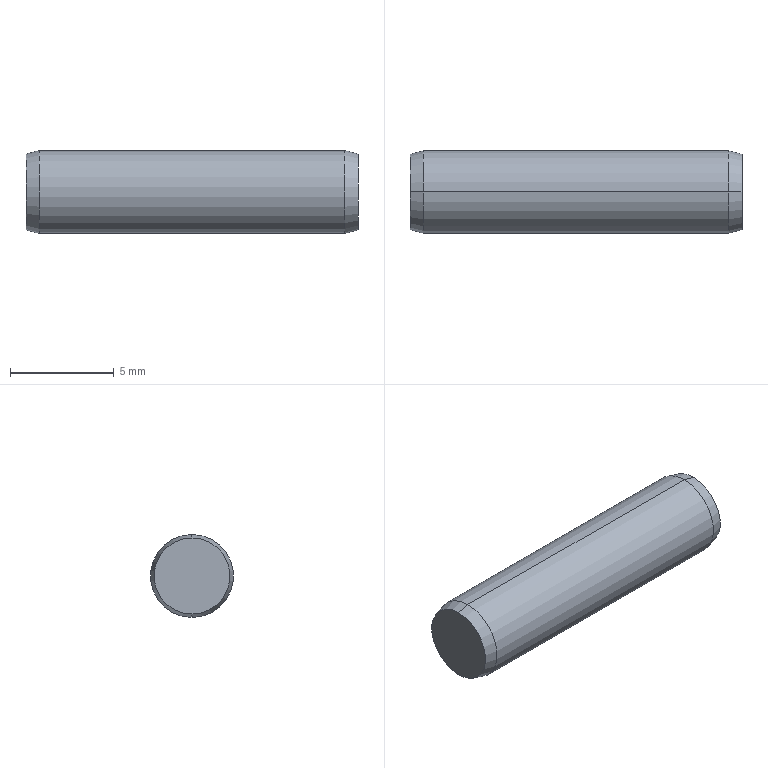Part | SolidWorks | features Revolution 1 | 1 solid | 8 faces | box 16 x 4 x 4 mm | volume 199.763 mm3 | cone 4 | cylinder 2 | plane 2 | commonest cylinder face diameters 4 x2
STEP:
#1=CARTESIAN_POINT('',(13.74,0.,2.));
#2=VERTEX_POINT('',#1);
#3=CARTESIAN_POINT('',(13.74,0.,-2.));
#4=VERTEX_POINT('',#3);
#5=CARTESIAN_POINT('',(13.74,0.,0.));
#6=DIRECTION('',(-1.,0.,0.));
#7=DIRECTION('',(0.,0.,1.));
#8=AXIS2_PLACEMENT_3D('',#5,#6,#7);
#9=CIRCLE('',#8,2.);
#10=EDGE_CURVE('',#2,#4,#9,.T.);
#11=ORIENTED_EDGE('',*,*,#10,.T.);
#12=CARTESIAN_POINT('',(-1.,0.,-2.));
#13=VERTEX_POINT('',#12);
#14=CARTESIAN_POINT('',(0.,0.,-2.));
#15=DIRECTION('',(-1.,0.,0.));
#16=VECTOR('',#15,1000.);
#17=LINE('',#14,#16);
#18=EDGE_CURVE('',#4,#13,#17,.T.);
#19=ORIENTED_EDGE('',*,*,#18,.T.);
#20=CARTESIAN_POINT('',(-1.,0.,2.));
#21=VERTEX_POINT('',#20);
#22=CARTESIAN_POINT('',(-1.,0.,0.));
#23=DIRECTION('',(-1.,0.,0.));
#24=DIRECTION('',(0.,0.,1.));
#25=AXIS2_PLACEMENT_3D('',#22,#23,#24);
#26=CIRCLE('',#25,2.);
#27=EDGE_CURVE('',#21,#13,#26,.T.);
#28=ORIENTED_EDGE('',*,*,#27,.F.);
#29=CARTESIAN_POINT('',(0.,0.,2.));
#30=DIRECTION('',(-1.,0.,0.));
#31=VECTOR('',#30,1000.);
#32=LINE('',#29,#31);
#33=EDGE_CURVE('',#2,#21,#32,.T.);
#34=ORIENTED_EDGE('',*,*,#33,.F.);
#35=EDGE_LOOP('',(#11,#19,#28,#34));
#36=FACE_OUTER_BOUND('',#35,.T.);
#37=CARTESIAN_POINT('',(0.,0.,0.));
#38=DIRECTION('',(-1.,0.,0.));
#39=DIRECTION('',(0.,0.,1.));
#40=AXIS2_PLACEMENT_3D('',#37,#38,#39);
#41=CYLINDRICAL_SURFACE('',#40,2.);
#42=ADVANCED_FACE('',(#36),#41,.T.);
#43=CARTESIAN_POINT('',(-1.63,0.,1.831));
#44=VERTEX_POINT('',#43);
#45=CARTESIAN_POINT('',(-1.63,0.,-1.831));
#46=VERTEX_POINT('',#45);
#47=CARTESIAN_POINT('',(-1.63,0.,0.));
#48=DIRECTION('',(-1.,0.,0.));
#49=DIRECTION('',(0.,0.,1.));
#50=AXIS2_PLACEMENT_3D('',#47,#48,#49);
#51=CIRCLE('',#50,1.831);
#52=EDGE_CURVE('',#44,#46,#51,.T.);
#53=ORIENTED_EDGE('',*,*,#52,.F.);
#54=CARTESIAN_POINT('',(-1.,0.,2.));
#55=DIRECTION('',(0.9659,0.,0.2588));
#56=VECTOR('',#55,1000.);
#57=LINE('',#54,#56);
#58=EDGE_CURVE('',#44,#21,#57,.T.);
#59=ORIENTED_EDGE('',*,*,#58,.T.);
#60=ORIENTED_EDGE('',*,*,#27,.T.);
#61=CARTESIAN_POINT('',(-1.,0.,-2.));
#62=DIRECTION('',(0.9659,0.,-0.2588));
#63=VECTOR('',#62,1000.);
#64=LINE('',#61,#63);
#65=EDGE_CURVE('',#46,#13,#64,.T.);
#66=ORIENTED_EDGE('',*,*,#65,.F.);
#67=EDGE_LOOP('',(#53,#59,#60,#66));
#68=FACE_OUTER_BOUND('',#67,.T.);
#69=CARTESIAN_POINT('',(-1.,0.,0.));
#70=DIRECTION('',(1.,0.,0.));
#71=DIRECTION('',(0.,0.,-1.));
#72=AXIS2_PLACEMENT_3D('',#69,#70,#71);
#73=CONICAL_SURFACE('',#72,2.,0.2618);
#74=ADVANCED_FACE('',(#68),#73,.T.);
#75=CARTESIAN_POINT('',(14.37,0.,1.831));
#76=VERTEX_POINT('',#75);
#77=CARTESIAN_POINT('',(14.37,0.,-1.831));
#78=VERTEX_POINT('',#77);
#79=CARTESIAN_POINT('',(14.37,0.,0.));
#80=DIRECTION('',(-1.,0.,0.));
#81=DIRECTION('',(0.,0.,1.));
#82=AXIS2_PLACEMENT_3D('',#79,#80,#81);
#83=CIRCLE('',#82,1.831);
#84=EDGE_CURVE('',#76,#78,#83,.T.);
#85=ORIENTED_EDGE('',*,*,#84,.T.);
#86=CARTESIAN_POINT('',(14.37,0.,-1.831));
#87=DIRECTION('',(-0.9659,0.,-0.2588));
#88=VECTOR('',#87,1000.);
#89=LINE('',#86,#88);
#90=EDGE_CURVE('',#78,#4,#89,.T.);
#91=ORIENTED_EDGE('',*,*,#90,.T.);
#92=ORIENTED_EDGE('',*,*,#10,.F.);
#93=CARTESIAN_POINT('',(14.37,0.,1.831));
#94=DIRECTION('',(-0.9659,0.,0.2588));
#95=VECTOR('',#94,1000.);
#96=LINE('',#93,#95);
#97=EDGE_CURVE('',#76,#2,#96,.T.);
#98=ORIENTED_EDGE('',*,*,#97,.F.);
#99=EDGE_LOOP('',(#85,#91,#92,#98));
#100=FACE_OUTER_BOUND('',#99,.T.);
#101=CARTESIAN_POINT('',(14.37,0.,0.));
#102=DIRECTION('',(-1.,0.,0.));
#103=DIRECTION('',(0.,0.,1.));
#104=AXIS2_PLACEMENT_3D('',#101,#102,#103);
#105=CONICAL_SURFACE('',#104,1.831,0.2618);
#106=ADVANCED_FACE('',(#100),#105,.T.);
#107=ORIENTED_EDGE('',*,*,#90,.F.);
#108=CARTESIAN_POINT('',(14.37,0.,0.));
#109=DIRECTION('',(-1.,0.,0.));
#110=DIRECTION('',(0.,0.,1.));
#111=AXIS2_PLACEMENT_3D('',#108,#109,#110);
#112=CIRCLE('',#111,1.831);
#113=EDGE_CURVE('',#78,#76,#112,.T.);
#114=ORIENTED_EDGE('',*,*,#113,.T.);
#115=ORIENTED_EDGE('',*,*,#97,.T.);
#116=CARTESIAN_POINT('',(13.74,0.,0.));
#117=DIRECTION('',(-1.,0.,0.));
#118=DIRECTION('',(0.,0.,1.));
#119=AXIS2_PLACEMENT_3D('',#116,#117,#118);
#120=CIRCLE('',#119,2.);
#121=EDGE_CURVE('',#4,#2,#120,.T.);
#122=ORIENTED_EDGE('',*,*,#121,.F.);
#123=EDGE_LOOP('',(#107,#114,#115,#122));
#124=FACE_OUTER_BOUND('',#123,.T.);
#125=CARTESIAN_POINT('',(14.37,0.,0.));
#126=DIRECTION('',(-1.,0.,0.));
#127=DIRECTION('',(0.,0.,1.));
#128=AXIS2_PLACEMENT_3D('',#125,#126,#127);
#129=CONICAL_SURFACE('',#128,1.831,0.2618);
#130=ADVANCED_FACE('',(#124),#129,.T.);
#131=ORIENTED_EDGE('',*,*,#84,.F.);
#132=ORIENTED_EDGE('',*,*,#113,.F.);
#133=EDGE_LOOP('',(#131,#132));
#134=FACE_OUTER_BOUND('',#133,.T.);
#135=CARTESIAN_POINT('',(14.37,1.831,0.));
#136=DIRECTION('',(-1.,0.,0.));
#137=DIRECTION('',(0.,0.,1.));
#138=AXIS2_PLACEMENT_3D('',#135,#136,#137);
#139=PLANE('',#138);
#140=ADVANCED_FACE('',(#134),#139,.F.);
#141=CARTESIAN_POINT('',(-1.63,0.,0.));
#142=DIRECTION('',(-1.,0.,0.));
#143=DIRECTION('',(0.,0.,1.));
#144=AXIS2_PLACEMENT_3D('',#141,#142,#143);
#145=CIRCLE('',#144,1.831);
#146=EDGE_CURVE('',#46,#44,#145,.T.);
#147=ORIENTED_EDGE('',*,*,#146,.T.);
#148=ORIENTED_EDGE('',*,*,#52,.T.);
#149=EDGE_LOOP('',(#147,#148));
#150=FACE_OUTER_BOUND('',#149,.T.);
#151=CARTESIAN_POINT('',(-1.63,1.831,0.));
#152=DIRECTION('',(1.,0.,0.));
#153=DIRECTION('',(0.,0.,-1.));
#154=AXIS2_PLACEMENT_3D('',#151,#152,#153);
#155=PLANE('',#154);
#156=ADVANCED_FACE('',(#150),#155,.F.);
#157=ORIENTED_EDGE('',*,*,#58,.F.);
#158=ORIENTED_EDGE('',*,*,#146,.F.);
#159=ORIENTED_EDGE('',*,*,#65,.T.);
#160=CARTESIAN_POINT('',(-1.,0.,0.));
#161=DIRECTION('',(-1.,0.,0.));
#162=DIRECTION('',(0.,0.,1.));
#163=AXIS2_PLACEMENT_3D('',#160,#161,#162);
#164=CIRCLE('',#163,2.);
#165=EDGE_CURVE('',#13,#21,#164,.T.);
#166=ORIENTED_EDGE('',*,*,#165,.T.);
#167=EDGE_LOOP('',(#157,#158,#159,#166));
#168=FACE_OUTER_BOUND('',#167,.T.);
#169=CARTESIAN_POINT('',(-1.,0.,0.));
#170=DIRECTION('',(1.,0.,0.));
#171=DIRECTION('',(0.,0.,-1.));
#172=AXIS2_PLACEMENT_3D('',#169,#170,#171);
#173=CONICAL_SURFACE('',#172,2.,0.2618);
#174=ADVANCED_FACE('',(#168),#173,.T.);
#175=ORIENTED_EDGE('',*,*,#18,.F.);
#176=ORIENTED_EDGE('',*,*,#121,.T.);
#177=ORIENTED_EDGE('',*,*,#33,.T.);
#178=ORIENTED_EDGE('',*,*,#165,.F.);
#179=EDGE_LOOP('',(#175,#176,#177,#178));
#180=FACE_OUTER_BOUND('',#179,.T.);
#181=CARTESIAN_POINT('',(0.,0.,0.));
#182=DIRECTION('',(-1.,0.,0.));
#183=DIRECTION('',(0.,0.,1.));
#184=AXIS2_PLACEMENT_3D('',#181,#182,#183);
#185=CYLINDRICAL_SURFACE('',#184,2.);
#186=ADVANCED_FACE('',(#180),#185,.T.);
#187=CLOSED_SHELL('',(#42,#74,#106,#130,#140,#156,#174,#186));
#188=MANIFOLD_SOLID_BREP('',#187);
#189=CARTESIAN_POINT('',(0.,0.,0.));
#190=DIRECTION('',(0.,0.,1.));
#191=DIRECTION('',(1.,0.,0.));
#192=AXIS2_PLACEMENT_3D('',#189,#190,#191);
#193=(LENGTH_UNIT()NAMED_UNIT(*)SI_UNIT(.MILLI.,.METRE.));
#194=UNCERTAINTY_MEASURE_WITH_UNIT(LENGTH_MEASURE(0.00001),#193,'','');
#195=(NAMED_UNIT(*)PLANE_ANGLE_UNIT()SI_UNIT($,.RADIAN.));
#196=(NAMED_UNIT(*)SI_UNIT($,.STERADIAN.)SOLID_ANGLE_UNIT());
#197=(GEOMETRIC_REPRESENTATION_CONTEXT(3)GLOBAL_UNCERTAINTY_ASSIGNED_CONTEXT((#194))GLOBAL_UNIT_ASSIGNED_CONTEXT((#193,#195,#196))REPRESENTATION_CONTEXT('',''));
#198=ADVANCED_BREP_SHAPE_REPRESENTATION('',(#188,#192),#197);